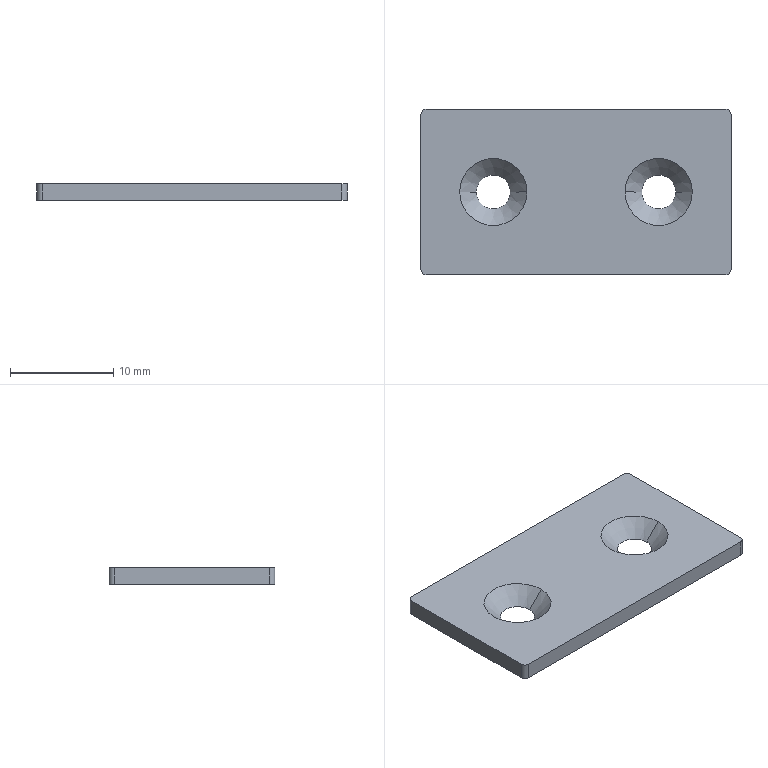Part | STEP file | Second C-100-B-2 Bracket Part [2] | 1 solid | 14 faces | box 30 x 16 x 1.6 mm | volume 705.168 mm3 | plane 6 | cone 4 | cylinder 4 | commonest cylinder face diameters 1 x4
STEP:
#1=CARTESIAN_POINT('',(9.65,8.,-1.6));
#2=VERTEX_POINT('',#1);
#3=CARTESIAN_POINT('',(6.35,8.,-1.6));
#4=VERTEX_POINT('',#3);
#5=CARTESIAN_POINT('',(8.,8.,-1.6));
#6=DIRECTION('',(0.,0.,-1.));
#7=DIRECTION('',(1.,0.,0.));
#8=AXIS2_PLACEMENT_3D('',#5,#6,#7);
#9=CIRCLE('',#8,1.65);
#10=EDGE_CURVE('',#2,#4,#9,.T.);
#11=ORIENTED_EDGE('',*,*,#10,.T.);
#12=CARTESIAN_POINT('',(4.75,8.,0.));
#13=VERTEX_POINT('',#12);
#14=CARTESIAN_POINT('',(4.75,8.,0.));
#15=DIRECTION('',(-0.7071,0.,0.7071));
#16=VECTOR('',#15,1000.);
#17=LINE('',#14,#16);
#18=EDGE_CURVE('',#4,#13,#17,.T.);
#19=ORIENTED_EDGE('',*,*,#18,.T.);
#20=CARTESIAN_POINT('',(11.25,8.,0.));
#21=VERTEX_POINT('',#20);
#22=CARTESIAN_POINT('',(8.,8.,0.));
#23=DIRECTION('',(0.,0.,-1.));
#24=DIRECTION('',(1.,0.,0.));
#25=AXIS2_PLACEMENT_3D('',#22,#23,#24);
#26=CIRCLE('',#25,3.25);
#27=EDGE_CURVE('',#21,#13,#26,.T.);
#28=ORIENTED_EDGE('',*,*,#27,.F.);
#29=CARTESIAN_POINT('',(11.25,8.,0.));
#30=DIRECTION('',(0.7071,0.,0.7071));
#31=VECTOR('',#30,1000.);
#32=LINE('',#29,#31);
#33=EDGE_CURVE('',#2,#21,#32,.T.);
#34=ORIENTED_EDGE('',*,*,#33,.F.);
#35=EDGE_LOOP('',(#11,#19,#28,#34));
#36=FACE_OUTER_BOUND('',#35,.T.);
#37=CARTESIAN_POINT('',(8.,8.,0.));
#38=DIRECTION('',(0.,0.,1.));
#39=DIRECTION('',(1.,0.,0.));
#40=AXIS2_PLACEMENT_3D('',#37,#38,#39);
#41=CONICAL_SURFACE('',#40,3.25,0.7854);
#42=ADVANCED_FACE('',(#36),#41,.F.);
#43=CARTESIAN_POINT('',(-6.35,8.,-1.6));
#44=VERTEX_POINT('',#43);
#45=CARTESIAN_POINT('',(-9.65,8.,-1.6));
#46=VERTEX_POINT('',#45);
#47=CARTESIAN_POINT('',(-8.,8.,-1.6));
#48=DIRECTION('',(0.,0.,-1.));
#49=DIRECTION('',(1.,0.,0.));
#50=AXIS2_PLACEMENT_3D('',#47,#48,#49);
#51=CIRCLE('',#50,1.65);
#52=EDGE_CURVE('',#44,#46,#51,.T.);
#53=ORIENTED_EDGE('',*,*,#52,.T.);
#54=CARTESIAN_POINT('',(-11.25,8.,0.));
#55=VERTEX_POINT('',#54);
#56=CARTESIAN_POINT('',(-11.25,8.,0.));
#57=DIRECTION('',(-0.7071,0.,0.7071));
#58=VECTOR('',#57,1000.);
#59=LINE('',#56,#58);
#60=EDGE_CURVE('',#46,#55,#59,.T.);
#61=ORIENTED_EDGE('',*,*,#60,.T.);
#62=CARTESIAN_POINT('',(-4.75,8.,0.));
#63=VERTEX_POINT('',#62);
#64=CARTESIAN_POINT('',(-8.,8.,0.));
#65=DIRECTION('',(0.,0.,-1.));
#66=DIRECTION('',(1.,0.,0.));
#67=AXIS2_PLACEMENT_3D('',#64,#65,#66);
#68=CIRCLE('',#67,3.25);
#69=EDGE_CURVE('',#63,#55,#68,.T.);
#70=ORIENTED_EDGE('',*,*,#69,.F.);
#71=CARTESIAN_POINT('',(-4.75,8.,0.));
#72=DIRECTION('',(0.7071,0.,0.7071));
#73=VECTOR('',#72,1000.);
#74=LINE('',#71,#73);
#75=EDGE_CURVE('',#44,#63,#74,.T.);
#76=ORIENTED_EDGE('',*,*,#75,.F.);
#77=EDGE_LOOP('',(#53,#61,#70,#76));
#78=FACE_OUTER_BOUND('',#77,.T.);
#79=CARTESIAN_POINT('',(-8.,8.,0.));
#80=DIRECTION('',(0.,0.,1.));
#81=DIRECTION('',(1.,0.,0.));
#82=AXIS2_PLACEMENT_3D('',#79,#80,#81);
#83=CONICAL_SURFACE('',#82,3.25,0.7854);
#84=ADVANCED_FACE('',(#78),#83,.F.);
#85=CARTESIAN_POINT('',(15.,0.5,-1.6));
#86=VERTEX_POINT('',#85);
#87=CARTESIAN_POINT('',(15.,15.5,-1.6));
#88=VERTEX_POINT('',#87);
#89=CARTESIAN_POINT('',(15.,15.5,-1.6));
#90=DIRECTION('',(0.,1.,0.));
#91=VECTOR('',#90,1000.);
#92=LINE('',#89,#91);
#93=EDGE_CURVE('',#86,#88,#92,.T.);
#94=ORIENTED_EDGE('',*,*,#93,.F.);
#95=CARTESIAN_POINT('',(14.5,0.,-1.6));
#96=VERTEX_POINT('',#95);
#97=CARTESIAN_POINT('',(14.5,0.5,-1.6));
#98=DIRECTION('',(0.,0.,1.));
#99=DIRECTION('',(1.,0.,0.));
#100=AXIS2_PLACEMENT_3D('',#97,#98,#99);
#101=CIRCLE('',#100,0.5);
#102=EDGE_CURVE('',#96,#86,#101,.T.);
#103=ORIENTED_EDGE('',*,*,#102,.F.);
#104=CARTESIAN_POINT('',(-14.5,0.,-1.6));
#105=VERTEX_POINT('',#104);
#106=CARTESIAN_POINT('',(14.5,0.,-1.6));
#107=DIRECTION('',(1.,0.,0.));
#108=VECTOR('',#107,1000.);
#109=LINE('',#106,#108);
#110=EDGE_CURVE('',#105,#96,#109,.T.);
#111=ORIENTED_EDGE('',*,*,#110,.F.);
#112=CARTESIAN_POINT('',(-15.,0.5,-1.6));
#113=VERTEX_POINT('',#112);
#114=CARTESIAN_POINT('',(-14.5,0.5,-1.6));
#115=DIRECTION('',(0.,0.,1.));
#116=DIRECTION('',(1.,0.,0.));
#117=AXIS2_PLACEMENT_3D('',#114,#115,#116);
#118=CIRCLE('',#117,0.5);
#119=EDGE_CURVE('',#113,#105,#118,.T.);
#120=ORIENTED_EDGE('',*,*,#119,.F.);
#121=CARTESIAN_POINT('',(-15.,15.5,-1.6));
#122=VERTEX_POINT('',#121);
#123=CARTESIAN_POINT('',(-15.,15.5,-1.6));
#124=DIRECTION('',(0.,-1.,0.));
#125=VECTOR('',#124,1000.);
#126=LINE('',#123,#125);
#127=EDGE_CURVE('',#122,#113,#126,.T.);
#128=ORIENTED_EDGE('',*,*,#127,.F.);
#129=CARTESIAN_POINT('',(-14.5,16.,-1.6));
#130=VERTEX_POINT('',#129);
#131=CARTESIAN_POINT('',(-14.5,15.5,-1.6));
#132=DIRECTION('',(0.,0.,1.));
#133=DIRECTION('',(1.,0.,0.));
#134=AXIS2_PLACEMENT_3D('',#131,#132,#133);
#135=CIRCLE('',#134,0.5);
#136=EDGE_CURVE('',#130,#122,#135,.T.);
#137=ORIENTED_EDGE('',*,*,#136,.F.);
#138=CARTESIAN_POINT('',(14.5,16.,-1.6));
#139=VERTEX_POINT('',#138);
#140=CARTESIAN_POINT('',(14.5,16.,-1.6));
#141=DIRECTION('',(-1.,0.,0.));
#142=VECTOR('',#141,1000.);
#143=LINE('',#140,#142);
#144=EDGE_CURVE('',#139,#130,#143,.T.);
#145=ORIENTED_EDGE('',*,*,#144,.F.);
#146=CARTESIAN_POINT('',(14.5,15.5,-1.6));
#147=DIRECTION('',(0.,0.,1.));
#148=DIRECTION('',(1.,0.,0.));
#149=AXIS2_PLACEMENT_3D('',#146,#147,#148);
#150=CIRCLE('',#149,0.5);
#151=EDGE_CURVE('',#88,#139,#150,.T.);
#152=ORIENTED_EDGE('',*,*,#151,.F.);
#153=EDGE_LOOP('',(#94,#103,#111,#120,#128,#137,#145,#152));
#154=FACE_OUTER_BOUND('',#153,.T.);
#155=ORIENTED_EDGE('',*,*,#10,.F.);
#156=CARTESIAN_POINT('',(8.,8.,-1.6));
#157=DIRECTION('',(0.,0.,-1.));
#158=DIRECTION('',(1.,0.,0.));
#159=AXIS2_PLACEMENT_3D('',#156,#157,#158);
#160=CIRCLE('',#159,1.65);
#161=EDGE_CURVE('',#4,#2,#160,.T.);
#162=ORIENTED_EDGE('',*,*,#161,.F.);
#163=EDGE_LOOP('',(#155,#162));
#164=FACE_BOUND('',#163,.T.);
#165=ORIENTED_EDGE('',*,*,#52,.F.);
#166=CARTESIAN_POINT('',(-8.,8.,-1.6));
#167=DIRECTION('',(0.,0.,-1.));
#168=DIRECTION('',(1.,0.,0.));
#169=AXIS2_PLACEMENT_3D('',#166,#167,#168);
#170=CIRCLE('',#169,1.65);
#171=EDGE_CURVE('',#46,#44,#170,.T.);
#172=ORIENTED_EDGE('',*,*,#171,.F.);
#173=EDGE_LOOP('',(#165,#172));
#174=FACE_BOUND('',#173,.T.);
#175=CARTESIAN_POINT('',(14.5,15.5,-1.6));
#176=DIRECTION('',(0.,0.,1.));
#177=DIRECTION('',(1.,0.,0.));
#178=AXIS2_PLACEMENT_3D('',#175,#176,#177);
#179=PLANE('',#178);
#180=ADVANCED_FACE('',(#154,#164,#174),#179,.F.);
#181=ORIENTED_EDGE('',*,*,#93,.T.);
#182=CARTESIAN_POINT('',(15.,15.5,0.));
#183=VERTEX_POINT('',#182);
#184=CARTESIAN_POINT('',(15.,15.5,-1.6));
#185=DIRECTION('',(0.,0.,1.));
#186=VECTOR('',#185,1000.);
#187=LINE('',#184,#186);
#188=EDGE_CURVE('',#88,#183,#187,.T.);
#189=ORIENTED_EDGE('',*,*,#188,.T.);
#190=CARTESIAN_POINT('',(15.,0.5,0.));
#191=VERTEX_POINT('',#190);
#192=CARTESIAN_POINT('',(15.,0.5,0.));
#193=DIRECTION('',(0.,-1.,0.));
#194=VECTOR('',#193,1000.);
#195=LINE('',#192,#194);
#196=EDGE_CURVE('',#183,#191,#195,.T.);
#197=ORIENTED_EDGE('',*,*,#196,.T.);
#198=CARTESIAN_POINT('',(15.,0.5,-1.6));
#199=DIRECTION('',(0.,0.,-1.));
#200=VECTOR('',#199,1000.);
#201=LINE('',#198,#200);
#202=EDGE_CURVE('',#191,#86,#201,.T.);
#203=ORIENTED_EDGE('',*,*,#202,.T.);
#204=EDGE_LOOP('',(#181,#189,#197,#203));
#205=FACE_OUTER_BOUND('',#204,.T.);
#206=CARTESIAN_POINT('',(15.,0.5,-1.6));
#207=DIRECTION('',(1.,0.,0.));
#208=DIRECTION('',(0.,0.,-1.));
#209=AXIS2_PLACEMENT_3D('',#206,#207,#208);
#210=PLANE('',#209);
#211=ADVANCED_FACE('',(#205),#210,.T.);
#212=ORIENTED_EDGE('',*,*,#110,.T.);
#213=CARTESIAN_POINT('',(14.5,0.,0.));
#214=VERTEX_POINT('',#213);
#215=CARTESIAN_POINT('',(14.5,0.,-1.6));
#216=DIRECTION('',(0.,0.,1.));
#217=VECTOR('',#216,1000.);
#218=LINE('',#215,#217);
#219=EDGE_CURVE('',#96,#214,#218,.T.);
#220=ORIENTED_EDGE('',*,*,#219,.T.);
#221=CARTESIAN_POINT('',(-14.5,0.,0.));
#222=VERTEX_POINT('',#221);
#223=CARTESIAN_POINT('',(-14.5,0.,0.));
#224=DIRECTION('',(-1.,0.,0.));
#225=VECTOR('',#224,1000.);
#226=LINE('',#223,#225);
#227=EDGE_CURVE('',#214,#222,#226,.T.);
#228=ORIENTED_EDGE('',*,*,#227,.T.);
#229=CARTESIAN_POINT('',(-14.5,0.,-1.6));
#230=DIRECTION('',(0.,0.,-1.));
#231=VECTOR('',#230,1000.);
#232=LINE('',#229,#231);
#233=EDGE_CURVE('',#222,#105,#232,.T.);
#234=ORIENTED_EDGE('',*,*,#233,.T.);
#235=EDGE_LOOP('',(#212,#220,#228,#234));
#236=FACE_OUTER_BOUND('',#235,.T.);
#237=CARTESIAN_POINT('',(-14.5,0.,-1.6));
#238=DIRECTION('',(0.,-1.,0.));
#239=DIRECTION('',(0.,0.,-1.));
#240=AXIS2_PLACEMENT_3D('',#237,#238,#239);
#241=PLANE('',#240);
#242=ADVANCED_FACE('',(#236),#241,.T.);
#243=ORIENTED_EDGE('',*,*,#127,.T.);
#244=CARTESIAN_POINT('',(-15.,0.5,0.));
#245=VERTEX_POINT('',#244);
#246=CARTESIAN_POINT('',(-15.,0.5,-1.6));
#247=DIRECTION('',(0.,0.,1.));
#248=VECTOR('',#247,1000.);
#249=LINE('',#246,#248);
#250=EDGE_CURVE('',#113,#245,#249,.T.);
#251=ORIENTED_EDGE('',*,*,#250,.T.);
#252=CARTESIAN_POINT('',(-15.,15.5,0.));
#253=VERTEX_POINT('',#252);
#254=CARTESIAN_POINT('',(-15.,15.5,0.));
#255=DIRECTION('',(0.,1.,0.));
#256=VECTOR('',#255,1000.);
#257=LINE('',#254,#256);
#258=EDGE_CURVE('',#245,#253,#257,.T.);
#259=ORIENTED_EDGE('',*,*,#258,.T.);
#260=CARTESIAN_POINT('',(-15.,15.5,-1.6));
#261=DIRECTION('',(0.,0.,-1.));
#262=VECTOR('',#261,1000.);
#263=LINE('',#260,#262);
#264=EDGE_CURVE('',#253,#122,#263,.T.);
#265=ORIENTED_EDGE('',*,*,#264,.T.);
#266=EDGE_LOOP('',(#243,#251,#259,#265));
#267=FACE_OUTER_BOUND('',#266,.T.);
#268=CARTESIAN_POINT('',(-15.,15.5,-1.6));
#269=DIRECTION('',(-1.,0.,0.));
#270=DIRECTION('',(0.,-1.,0.));
#271=AXIS2_PLACEMENT_3D('',#268,#269,#270);
#272=PLANE('',#271);
#273=ADVANCED_FACE('',(#267),#272,.T.);
#274=ORIENTED_EDGE('',*,*,#144,.T.);
#275=CARTESIAN_POINT('',(-14.5,16.,0.));
#276=VERTEX_POINT('',#275);
#277=CARTESIAN_POINT('',(-14.5,16.,-1.6));
#278=DIRECTION('',(0.,0.,1.));
#279=VECTOR('',#278,1000.);
#280=LINE('',#277,#279);
#281=EDGE_CURVE('',#130,#276,#280,.T.);
#282=ORIENTED_EDGE('',*,*,#281,.T.);
#283=CARTESIAN_POINT('',(14.5,16.,0.));
#284=VERTEX_POINT('',#283);
#285=CARTESIAN_POINT('',(14.5,16.,0.));
#286=DIRECTION('',(1.,0.,0.));
#287=VECTOR('',#286,1000.);
#288=LINE('',#285,#287);
#289=EDGE_CURVE('',#276,#284,#288,.T.);
#290=ORIENTED_EDGE('',*,*,#289,.T.);
#291=CARTESIAN_POINT('',(14.5,16.,-1.6));
#292=DIRECTION('',(0.,0.,-1.));
#293=VECTOR('',#292,1000.);
#294=LINE('',#291,#293);
#295=EDGE_CURVE('',#284,#139,#294,.T.);
#296=ORIENTED_EDGE('',*,*,#295,.T.);
#297=EDGE_LOOP('',(#274,#282,#290,#296));
#298=FACE_OUTER_BOUND('',#297,.T.);
#299=CARTESIAN_POINT('',(14.5,16.,-1.6));
#300=DIRECTION('',(0.,1.,0.));
#301=DIRECTION('',(-1.,0.,0.));
#302=AXIS2_PLACEMENT_3D('',#299,#300,#301);
#303=PLANE('',#302);
#304=ADVANCED_FACE('',(#298),#303,.T.);
#305=ORIENTED_EDGE('',*,*,#18,.F.);
#306=ORIENTED_EDGE('',*,*,#161,.T.);
#307=ORIENTED_EDGE('',*,*,#33,.T.);
#308=CARTESIAN_POINT('',(8.,8.,0.));
#309=DIRECTION('',(0.,0.,-1.));
#310=DIRECTION('',(1.,0.,0.));
#311=AXIS2_PLACEMENT_3D('',#308,#309,#310);
#312=CIRCLE('',#311,3.25);
#313=EDGE_CURVE('',#13,#21,#312,.T.);
#314=ORIENTED_EDGE('',*,*,#313,.F.);
#315=EDGE_LOOP('',(#305,#306,#307,#314));
#316=FACE_OUTER_BOUND('',#315,.T.);
#317=CARTESIAN_POINT('',(8.,8.,0.));
#318=DIRECTION('',(0.,0.,1.));
#319=DIRECTION('',(1.,0.,0.));
#320=AXIS2_PLACEMENT_3D('',#317,#318,#319);
#321=CONICAL_SURFACE('',#320,3.25,0.7854);
#322=ADVANCED_FACE('',(#316),#321,.F.);
#323=ORIENTED_EDGE('',*,*,#60,.F.);
#324=ORIENTED_EDGE('',*,*,#171,.T.);
#325=ORIENTED_EDGE('',*,*,#75,.T.);
#326=CARTESIAN_POINT('',(-8.,8.,0.));
#327=DIRECTION('',(0.,0.,-1.));
#328=DIRECTION('',(1.,0.,0.));
#329=AXIS2_PLACEMENT_3D('',#326,#327,#328);
#330=CIRCLE('',#329,3.25);
#331=EDGE_CURVE('',#55,#63,#330,.T.);
#332=ORIENTED_EDGE('',*,*,#331,.F.);
#333=EDGE_LOOP('',(#323,#324,#325,#332));
#334=FACE_OUTER_BOUND('',#333,.T.);
#335=CARTESIAN_POINT('',(-8.,8.,0.));
#336=DIRECTION('',(0.,0.,1.));
#337=DIRECTION('',(1.,0.,0.));
#338=AXIS2_PLACEMENT_3D('',#335,#336,#337);
#339=CONICAL_SURFACE('',#338,3.25,0.7854);
#340=ADVANCED_FACE('',(#334),#339,.F.);
#341=ORIENTED_EDGE('',*,*,#151,.T.);
#342=ORIENTED_EDGE('',*,*,#295,.F.);
#343=CARTESIAN_POINT('',(14.5,15.5,0.));
#344=DIRECTION('',(0.,0.,-1.));
#345=DIRECTION('',(1.,0.,0.));
#346=AXIS2_PLACEMENT_3D('',#343,#344,#345);
#347=CIRCLE('',#346,0.5);
#348=EDGE_CURVE('',#284,#183,#347,.T.);
#349=ORIENTED_EDGE('',*,*,#348,.T.);
#350=ORIENTED_EDGE('',*,*,#188,.F.);
#351=EDGE_LOOP('',(#341,#342,#349,#350));
#352=FACE_OUTER_BOUND('',#351,.T.);
#353=CARTESIAN_POINT('',(14.5,15.5,-1.6));
#354=DIRECTION('',(0.,0.,1.));
#355=DIRECTION('',(1.,0.,0.));
#356=AXIS2_PLACEMENT_3D('',#353,#354,#355);
#357=CYLINDRICAL_SURFACE('',#356,0.5);
#358=ADVANCED_FACE('',(#352),#357,.T.);
#359=ORIENTED_EDGE('',*,*,#102,.T.);
#360=ORIENTED_EDGE('',*,*,#202,.F.);
#361=CARTESIAN_POINT('',(14.5,0.5,0.));
#362=DIRECTION('',(0.,0.,-1.));
#363=DIRECTION('',(1.,0.,0.));
#364=AXIS2_PLACEMENT_3D('',#361,#362,#363);
#365=CIRCLE('',#364,0.5);
#366=EDGE_CURVE('',#191,#214,#365,.T.);
#367=ORIENTED_EDGE('',*,*,#366,.T.);
#368=ORIENTED_EDGE('',*,*,#219,.F.);
#369=EDGE_LOOP('',(#359,#360,#367,#368));
#370=FACE_OUTER_BOUND('',#369,.T.);
#371=CARTESIAN_POINT('',(14.5,0.5,-1.6));
#372=DIRECTION('',(0.,0.,1.));
#373=DIRECTION('',(1.,0.,0.));
#374=AXIS2_PLACEMENT_3D('',#371,#372,#373);
#375=CYLINDRICAL_SURFACE('',#374,0.5);
#376=ADVANCED_FACE('',(#370),#375,.T.);
#377=ORIENTED_EDGE('',*,*,#366,.F.);
#378=ORIENTED_EDGE('',*,*,#196,.F.);
#379=ORIENTED_EDGE('',*,*,#348,.F.);
#380=ORIENTED_EDGE('',*,*,#289,.F.);
#381=CARTESIAN_POINT('',(-14.5,15.5,0.));
#382=DIRECTION('',(0.,0.,1.));
#383=DIRECTION('',(1.,0.,0.));
#384=AXIS2_PLACEMENT_3D('',#381,#382,#383);
#385=CIRCLE('',#384,0.5);
#386=EDGE_CURVE('',#276,#253,#385,.T.);
#387=ORIENTED_EDGE('',*,*,#386,.T.);
#388=ORIENTED_EDGE('',*,*,#258,.F.);
#389=CARTESIAN_POINT('',(-14.5,0.5,0.));
#390=DIRECTION('',(0.,0.,1.));
#391=DIRECTION('',(1.,0.,0.));
#392=AXIS2_PLACEMENT_3D('',#389,#390,#391);
#393=CIRCLE('',#392,0.5);
#394=EDGE_CURVE('',#245,#222,#393,.T.);
#395=ORIENTED_EDGE('',*,*,#394,.T.);
#396=ORIENTED_EDGE('',*,*,#227,.F.);
#397=EDGE_LOOP('',(#377,#378,#379,#380,#387,#388,#395,#396));
#398=FACE_OUTER_BOUND('',#397,.T.);
#399=ORIENTED_EDGE('',*,*,#27,.T.);
#400=ORIENTED_EDGE('',*,*,#313,.T.);
#401=EDGE_LOOP('',(#399,#400));
#402=FACE_BOUND('',#401,.T.);
#403=ORIENTED_EDGE('',*,*,#69,.T.);
#404=ORIENTED_EDGE('',*,*,#331,.T.);
#405=EDGE_LOOP('',(#403,#404));
#406=FACE_BOUND('',#405,.T.);
#407=CARTESIAN_POINT('',(14.5,15.5,0.));
#408=DIRECTION('',(0.,0.,1.));
#409=DIRECTION('',(1.,0.,0.));
#410=AXIS2_PLACEMENT_3D('',#407,#408,#409);
#411=PLANE('',#410);
#412=ADVANCED_FACE('',(#398,#402,#406),#411,.T.);
#413=ORIENTED_EDGE('',*,*,#119,.T.);
#414=ORIENTED_EDGE('',*,*,#233,.F.);
#415=ORIENTED_EDGE('',*,*,#394,.F.);
#416=ORIENTED_EDGE('',*,*,#250,.F.);
#417=EDGE_LOOP('',(#413,#414,#415,#416));
#418=FACE_OUTER_BOUND('',#417,.T.);
#419=CARTESIAN_POINT('',(-14.5,0.5,-1.6));
#420=DIRECTION('',(0.,0.,1.));
#421=DIRECTION('',(1.,0.,0.));
#422=AXIS2_PLACEMENT_3D('',#419,#420,#421);
#423=CYLINDRICAL_SURFACE('',#422,0.5);
#424=ADVANCED_FACE('',(#418),#423,.T.);
#425=ORIENTED_EDGE('',*,*,#136,.T.);
#426=ORIENTED_EDGE('',*,*,#264,.F.);
#427=ORIENTED_EDGE('',*,*,#386,.F.);
#428=ORIENTED_EDGE('',*,*,#281,.F.);
#429=EDGE_LOOP('',(#425,#426,#427,#428));
#430=FACE_OUTER_BOUND('',#429,.T.);
#431=CARTESIAN_POINT('',(-14.5,15.5,-1.6));
#432=DIRECTION('',(0.,0.,1.));
#433=DIRECTION('',(1.,0.,0.));
#434=AXIS2_PLACEMENT_3D('',#431,#432,#433);
#435=CYLINDRICAL_SURFACE('',#434,0.5);
#436=ADVANCED_FACE('',(#430),#435,.T.);
#437=CLOSED_SHELL('',(#42,#84,#180,#211,#242,#273,#304,#322,#340,#358,#376,#412,#424,#436));
#438=MANIFOLD_SOLID_BREP('',#437);
#439=CARTESIAN_POINT('',(0.,0.,0.));
#440=DIRECTION('',(0.,0.,1.));
#441=DIRECTION('',(1.,0.,0.));
#442=AXIS2_PLACEMENT_3D('',#439,#440,#441);
#443=(LENGTH_UNIT()NAMED_UNIT(*)SI_UNIT(.MILLI.,.METRE.));
#444=UNCERTAINTY_MEASURE_WITH_UNIT(LENGTH_MEASURE(0.00001),#443,'','');
#445=(NAMED_UNIT(*)PLANE_ANGLE_UNIT()SI_UNIT($,.RADIAN.));
#446=(NAMED_UNIT(*)SI_UNIT($,.STERADIAN.)SOLID_ANGLE_UNIT());
#447=(GEOMETRIC_REPRESENTATION_CONTEXT(3)GLOBAL_UNCERTAINTY_ASSIGNED_CONTEXT((#444))GLOBAL_UNIT_ASSIGNED_CONTEXT((#443,#445,#446))REPRESENTATION_CONTEXT('',''));
#448=ADVANCED_BREP_SHAPE_REPRESENTATION('',(#438,#442),#447);